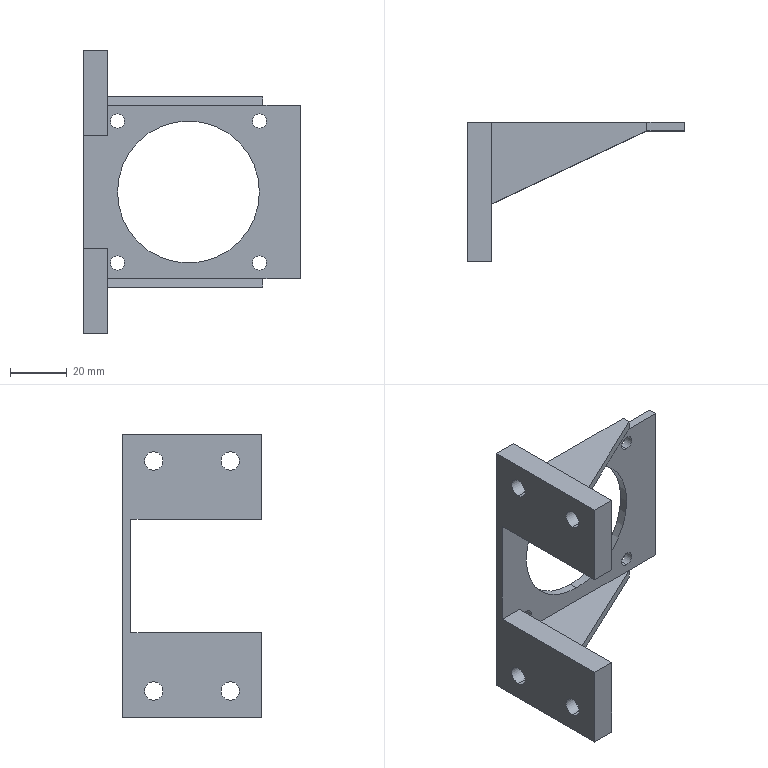Part | SolidWorks | features ICE 5, Extrusion 1, MirrorPattern 1 | 1 solid | 40 faces | box 76.5 x 49 x 100 mm | volume 36422 mm3 | plane 22 | cylinder 18 | commonest cylinder face diameters 5 x8 6.5 x8 50 x2
STEP:
#1=CARTESIAN_POINT('',(12.,24.5,-22.5));
#2=VERTEX_POINT('',#1);
#3=CARTESIAN_POINT('',(12.,24.5,-27.5));
#4=VERTEX_POINT('',#3);
#5=CARTESIAN_POINT('',(12.,24.5,-25.));
#6=DIRECTION('',(0.,-1.,0.));
#7=DIRECTION('',(0.,0.,-1.));
#8=AXIS2_PLACEMENT_3D('',#5,#6,#7);
#9=CIRCLE('',#8,2.5);
#10=EDGE_CURVE('',#2,#4,#9,.T.);
#11=ORIENTED_EDGE('',*,*,#10,.F.);
#12=CARTESIAN_POINT('',(12.,21.5,-22.5));
#13=VERTEX_POINT('',#12);
#14=CARTESIAN_POINT('',(12.,89.5,-22.5));
#15=DIRECTION('',(0.,-1.,0.));
#16=VECTOR('',#15,1000.);
#17=LINE('',#14,#16);
#18=EDGE_CURVE('',#2,#13,#17,.T.);
#19=ORIENTED_EDGE('',*,*,#18,.T.);
#20=CARTESIAN_POINT('',(12.,21.5,-27.5));
#21=VERTEX_POINT('',#20);
#22=CARTESIAN_POINT('',(12.,21.5,-25.));
#23=DIRECTION('',(0.,-1.,0.));
#24=DIRECTION('',(0.,0.,-1.));
#25=AXIS2_PLACEMENT_3D('',#22,#23,#24);
#26=CIRCLE('',#25,2.5);
#27=EDGE_CURVE('',#13,#21,#26,.T.);
#28=ORIENTED_EDGE('',*,*,#27,.T.);
#29=CARTESIAN_POINT('',(12.,89.5,-27.5));
#30=DIRECTION('',(0.,-1.,0.));
#31=VECTOR('',#30,1000.);
#32=LINE('',#29,#31);
#33=EDGE_CURVE('',#4,#21,#32,.T.);
#34=ORIENTED_EDGE('',*,*,#33,.F.);
#35=EDGE_LOOP('',(#11,#19,#28,#34));
#36=FACE_OUTER_BOUND('',#35,.T.);
#37=CARTESIAN_POINT('',(12.,89.5,-25.));
#38=DIRECTION('',(0.,-1.,0.));
#39=DIRECTION('',(0.,0.,-1.));
#40=AXIS2_PLACEMENT_3D('',#37,#38,#39);
#41=CYLINDRICAL_SURFACE('',#40,2.5);
#42=ADVANCED_FACE('',(#36),#41,.F.);
#43=CARTESIAN_POINT('',(62.,24.5,-22.5));
#44=VERTEX_POINT('',#43);
#45=CARTESIAN_POINT('',(62.,24.5,-27.5));
#46=VERTEX_POINT('',#45);
#47=CARTESIAN_POINT('',(62.,24.5,-25.));
#48=DIRECTION('',(0.,-1.,0.));
#49=DIRECTION('',(0.,0.,-1.));
#50=AXIS2_PLACEMENT_3D('',#47,#48,#49);
#51=CIRCLE('',#50,2.5);
#52=EDGE_CURVE('',#44,#46,#51,.T.);
#53=ORIENTED_EDGE('',*,*,#52,.F.);
#54=CARTESIAN_POINT('',(62.,21.5,-22.5));
#55=VERTEX_POINT('',#54);
#56=CARTESIAN_POINT('',(62.,89.5,-22.5));
#57=DIRECTION('',(0.,-1.,0.));
#58=VECTOR('',#57,1000.);
#59=LINE('',#56,#58);
#60=EDGE_CURVE('',#44,#55,#59,.T.);
#61=ORIENTED_EDGE('',*,*,#60,.T.);
#62=CARTESIAN_POINT('',(62.,21.5,-27.5));
#63=VERTEX_POINT('',#62);
#64=CARTESIAN_POINT('',(62.,21.5,-25.));
#65=DIRECTION('',(0.,-1.,0.));
#66=DIRECTION('',(0.,0.,-1.));
#67=AXIS2_PLACEMENT_3D('',#64,#65,#66);
#68=CIRCLE('',#67,2.5);
#69=EDGE_CURVE('',#55,#63,#68,.T.);
#70=ORIENTED_EDGE('',*,*,#69,.T.);
#71=CARTESIAN_POINT('',(62.,89.5,-27.5));
#72=DIRECTION('',(0.,-1.,0.));
#73=VECTOR('',#72,1000.);
#74=LINE('',#71,#73);
#75=EDGE_CURVE('',#46,#63,#74,.T.);
#76=ORIENTED_EDGE('',*,*,#75,.F.);
#77=EDGE_LOOP('',(#53,#61,#70,#76));
#78=FACE_OUTER_BOUND('',#77,.T.);
#79=CARTESIAN_POINT('',(62.,89.5,-25.));
#80=DIRECTION('',(0.,-1.,0.));
#81=DIRECTION('',(0.,0.,-1.));
#82=AXIS2_PLACEMENT_3D('',#79,#80,#81);
#83=CYLINDRICAL_SURFACE('',#82,2.5);
#84=ADVANCED_FACE('',(#78),#83,.F.);
#85=CARTESIAN_POINT('',(62.,24.5,27.5));
#86=VERTEX_POINT('',#85);
#87=CARTESIAN_POINT('',(62.,24.5,22.5));
#88=VERTEX_POINT('',#87);
#89=CARTESIAN_POINT('',(62.,24.5,25.));
#90=DIRECTION('',(0.,-1.,0.));
#91=DIRECTION('',(0.,0.,-1.));
#92=AXIS2_PLACEMENT_3D('',#89,#90,#91);
#93=CIRCLE('',#92,2.5);
#94=EDGE_CURVE('',#86,#88,#93,.T.);
#95=ORIENTED_EDGE('',*,*,#94,.F.);
#96=CARTESIAN_POINT('',(62.,21.5,27.5));
#97=VERTEX_POINT('',#96);
#98=CARTESIAN_POINT('',(62.,89.5,27.5));
#99=DIRECTION('',(0.,-1.,0.));
#100=VECTOR('',#99,1000.);
#101=LINE('',#98,#100);
#102=EDGE_CURVE('',#86,#97,#101,.T.);
#103=ORIENTED_EDGE('',*,*,#102,.T.);
#104=CARTESIAN_POINT('',(62.,21.5,22.5));
#105=VERTEX_POINT('',#104);
#106=CARTESIAN_POINT('',(62.,21.5,25.));
#107=DIRECTION('',(0.,-1.,0.));
#108=DIRECTION('',(0.,0.,-1.));
#109=AXIS2_PLACEMENT_3D('',#106,#107,#108);
#110=CIRCLE('',#109,2.5);
#111=EDGE_CURVE('',#97,#105,#110,.T.);
#112=ORIENTED_EDGE('',*,*,#111,.T.);
#113=CARTESIAN_POINT('',(62.,89.5,22.5));
#114=DIRECTION('',(0.,-1.,0.));
#115=VECTOR('',#114,1000.);
#116=LINE('',#113,#115);
#117=EDGE_CURVE('',#88,#105,#116,.T.);
#118=ORIENTED_EDGE('',*,*,#117,.F.);
#119=EDGE_LOOP('',(#95,#103,#112,#118));
#120=FACE_OUTER_BOUND('',#119,.T.);
#121=CARTESIAN_POINT('',(62.,89.5,25.));
#122=DIRECTION('',(0.,-1.,0.));
#123=DIRECTION('',(0.,0.,-1.));
#124=AXIS2_PLACEMENT_3D('',#121,#122,#123);
#125=CYLINDRICAL_SURFACE('',#124,2.5);
#126=ADVANCED_FACE('',(#120),#125,.F.);
#127=CARTESIAN_POINT('',(12.,24.5,27.5));
#128=VERTEX_POINT('',#127);
#129=CARTESIAN_POINT('',(12.,24.5,22.5));
#130=VERTEX_POINT('',#129);
#131=CARTESIAN_POINT('',(12.,24.5,25.));
#132=DIRECTION('',(0.,-1.,0.));
#133=DIRECTION('',(0.,0.,-1.));
#134=AXIS2_PLACEMENT_3D('',#131,#132,#133);
#135=CIRCLE('',#134,2.5);
#136=EDGE_CURVE('',#128,#130,#135,.T.);
#137=ORIENTED_EDGE('',*,*,#136,.F.);
#138=CARTESIAN_POINT('',(12.,21.5,27.5));
#139=VERTEX_POINT('',#138);
#140=CARTESIAN_POINT('',(12.,89.5,27.5));
#141=DIRECTION('',(0.,-1.,0.));
#142=VECTOR('',#141,1000.);
#143=LINE('',#140,#142);
#144=EDGE_CURVE('',#128,#139,#143,.T.);
#145=ORIENTED_EDGE('',*,*,#144,.T.);
#146=CARTESIAN_POINT('',(12.,21.5,22.5));
#147=VERTEX_POINT('',#146);
#148=CARTESIAN_POINT('',(12.,21.5,25.));
#149=DIRECTION('',(0.,-1.,0.));
#150=DIRECTION('',(0.,0.,-1.));
#151=AXIS2_PLACEMENT_3D('',#148,#149,#150);
#152=CIRCLE('',#151,2.5);
#153=EDGE_CURVE('',#139,#147,#152,.T.);
#154=ORIENTED_EDGE('',*,*,#153,.T.);
#155=CARTESIAN_POINT('',(12.,89.5,22.5));
#156=DIRECTION('',(0.,-1.,0.));
#157=VECTOR('',#156,1000.);
#158=LINE('',#155,#157);
#159=EDGE_CURVE('',#130,#147,#158,.T.);
#160=ORIENTED_EDGE('',*,*,#159,.F.);
#161=EDGE_LOOP('',(#137,#145,#154,#160));
#162=FACE_OUTER_BOUND('',#161,.T.);
#163=CARTESIAN_POINT('',(12.,89.5,25.));
#164=DIRECTION('',(0.,-1.,0.));
#165=DIRECTION('',(0.,0.,-1.));
#166=AXIS2_PLACEMENT_3D('',#163,#164,#165);
#167=CYLINDRICAL_SURFACE('',#166,2.5);
#168=ADVANCED_FACE('',(#162),#167,.F.);
#169=CARTESIAN_POINT('',(37.,24.5,25.));
#170=VERTEX_POINT('',#169);
#171=CARTESIAN_POINT('',(37.,24.5,-25.));
#172=VERTEX_POINT('',#171);
#173=CARTESIAN_POINT('',(37.,24.5,0.));
#174=DIRECTION('',(0.,-1.,0.));
#175=DIRECTION('',(0.,0.,-1.));
#176=AXIS2_PLACEMENT_3D('',#173,#174,#175);
#177=CIRCLE('',#176,25.);
#178=EDGE_CURVE('',#170,#172,#177,.T.);
#179=ORIENTED_EDGE('',*,*,#178,.F.);
#180=CARTESIAN_POINT('',(37.,21.5,25.));
#181=VERTEX_POINT('',#180);
#182=CARTESIAN_POINT('',(37.,89.5,25.));
#183=DIRECTION('',(0.,-1.,0.));
#184=VECTOR('',#183,1000.);
#185=LINE('',#182,#184);
#186=EDGE_CURVE('',#170,#181,#185,.T.);
#187=ORIENTED_EDGE('',*,*,#186,.T.);
#188=CARTESIAN_POINT('',(37.,21.5,-25.));
#189=VERTEX_POINT('',#188);
#190=CARTESIAN_POINT('',(37.,21.5,0.));
#191=DIRECTION('',(0.,-1.,0.));
#192=DIRECTION('',(0.,0.,-1.));
#193=AXIS2_PLACEMENT_3D('',#190,#191,#192);
#194=CIRCLE('',#193,25.);
#195=EDGE_CURVE('',#181,#189,#194,.T.);
#196=ORIENTED_EDGE('',*,*,#195,.T.);
#197=CARTESIAN_POINT('',(37.,89.5,-25.));
#198=DIRECTION('',(0.,-1.,0.));
#199=VECTOR('',#198,1000.);
#200=LINE('',#197,#199);
#201=EDGE_CURVE('',#172,#189,#200,.T.);
#202=ORIENTED_EDGE('',*,*,#201,.F.);
#203=EDGE_LOOP('',(#179,#187,#196,#202));
#204=FACE_OUTER_BOUND('',#203,.T.);
#205=CARTESIAN_POINT('',(37.,89.5,0.));
#206=DIRECTION('',(0.,-1.,0.));
#207=DIRECTION('',(0.,0.,-1.));
#208=AXIS2_PLACEMENT_3D('',#205,#206,#207);
#209=CYLINDRICAL_SURFACE('',#208,25.);
#210=ADVANCED_FACE('',(#204),#209,.F.);
#211=CARTESIAN_POINT('',(8.5,-13.5,43.75));
#212=VERTEX_POINT('',#211);
#213=CARTESIAN_POINT('',(8.5,-13.5,37.25));
#214=VERTEX_POINT('',#213);
#215=CARTESIAN_POINT('',(8.5,-13.5,40.5));
#216=DIRECTION('',(1.,0.,0.));
#217=DIRECTION('',(0.,0.,-1.));
#218=AXIS2_PLACEMENT_3D('',#215,#216,#217);
#219=CIRCLE('',#218,3.25);
#220=EDGE_CURVE('',#212,#214,#219,.T.);
#221=ORIENTED_EDGE('',*,*,#220,.T.);
#222=CARTESIAN_POINT('',(0.,-13.5,37.25));
#223=VERTEX_POINT('',#222);
#224=CARTESIAN_POINT('',(8.5,-13.5,37.25));
#225=DIRECTION('',(-1.,0.,0.));
#226=VECTOR('',#225,1000.);
#227=LINE('',#224,#226);
#228=EDGE_CURVE('',#214,#223,#227,.T.);
#229=ORIENTED_EDGE('',*,*,#228,.T.);
#230=CARTESIAN_POINT('',(0.,-13.5,43.75));
#231=VERTEX_POINT('',#230);
#232=CARTESIAN_POINT('',(0.,-13.5,40.5));
#233=DIRECTION('',(1.,0.,0.));
#234=DIRECTION('',(0.,0.,-1.));
#235=AXIS2_PLACEMENT_3D('',#232,#233,#234);
#236=CIRCLE('',#235,3.25);
#237=EDGE_CURVE('',#231,#223,#236,.T.);
#238=ORIENTED_EDGE('',*,*,#237,.F.);
#239=CARTESIAN_POINT('',(8.5,-13.5,43.75));
#240=DIRECTION('',(-1.,0.,0.));
#241=VECTOR('',#240,1000.);
#242=LINE('',#239,#241);
#243=EDGE_CURVE('',#212,#231,#242,.T.);
#244=ORIENTED_EDGE('',*,*,#243,.F.);
#245=EDGE_LOOP('',(#221,#229,#238,#244));
#246=FACE_OUTER_BOUND('',#245,.T.);
#247=CARTESIAN_POINT('',(8.5,-13.5,40.5));
#248=DIRECTION('',(-1.,0.,0.));
#249=DIRECTION('',(0.,0.,1.));
#250=AXIS2_PLACEMENT_3D('',#247,#248,#249);
#251=CYLINDRICAL_SURFACE('',#250,3.25);
#252=ADVANCED_FACE('',(#246),#251,.F.);
#253=CARTESIAN_POINT('',(8.5,-13.5,-37.25));
#254=VERTEX_POINT('',#253);
#255=CARTESIAN_POINT('',(8.5,-13.5,-43.75));
#256=VERTEX_POINT('',#255);
#257=CARTESIAN_POINT('',(8.5,-13.5,-40.5));
#258=DIRECTION('',(1.,0.,0.));
#259=DIRECTION('',(0.,0.,-1.));
#260=AXIS2_PLACEMENT_3D('',#257,#258,#259);
#261=CIRCLE('',#260,3.25);
#262=EDGE_CURVE('',#254,#256,#261,.T.);
#263=ORIENTED_EDGE('',*,*,#262,.T.);
#264=CARTESIAN_POINT('',(0.,-13.5,-43.75));
#265=VERTEX_POINT('',#264);
#266=CARTESIAN_POINT('',(8.5,-13.5,-43.75));
#267=DIRECTION('',(-1.,0.,0.));
#268=VECTOR('',#267,1000.);
#269=LINE('',#266,#268);
#270=EDGE_CURVE('',#256,#265,#269,.T.);
#271=ORIENTED_EDGE('',*,*,#270,.T.);
#272=CARTESIAN_POINT('',(0.,-13.5,-37.25));
#273=VERTEX_POINT('',#272);
#274=CARTESIAN_POINT('',(0.,-13.5,-40.5));
#275=DIRECTION('',(1.,0.,0.));
#276=DIRECTION('',(0.,0.,-1.));
#277=AXIS2_PLACEMENT_3D('',#274,#275,#276);
#278=CIRCLE('',#277,3.25);
#279=EDGE_CURVE('',#273,#265,#278,.T.);
#280=ORIENTED_EDGE('',*,*,#279,.F.);
#281=CARTESIAN_POINT('',(8.5,-13.5,-37.25));
#282=DIRECTION('',(-1.,0.,0.));
#283=VECTOR('',#282,1000.);
#284=LINE('',#281,#283);
#285=EDGE_CURVE('',#254,#273,#284,.T.);
#286=ORIENTED_EDGE('',*,*,#285,.F.);
#287=EDGE_LOOP('',(#263,#271,#280,#286));
#288=FACE_OUTER_BOUND('',#287,.T.);
#289=CARTESIAN_POINT('',(8.5,-13.5,-40.5));
#290=DIRECTION('',(-1.,0.,0.));
#291=DIRECTION('',(0.,0.,1.));
#292=AXIS2_PLACEMENT_3D('',#289,#290,#291);
#293=CYLINDRICAL_SURFACE('',#292,3.25);
#294=ADVANCED_FACE('',(#288),#293,.F.);
#295=CARTESIAN_POINT('',(8.5,13.5,-37.25));
#296=VERTEX_POINT('',#295);
#297=CARTESIAN_POINT('',(8.5,13.5,-43.75));
#298=VERTEX_POINT('',#297);
#299=CARTESIAN_POINT('',(8.5,13.5,-40.5));
#300=DIRECTION('',(1.,0.,0.));
#301=DIRECTION('',(0.,0.,-1.));
#302=AXIS2_PLACEMENT_3D('',#299,#300,#301);
#303=CIRCLE('',#302,3.25);
#304=EDGE_CURVE('',#296,#298,#303,.T.);
#305=ORIENTED_EDGE('',*,*,#304,.T.);
#306=CARTESIAN_POINT('',(0.,13.5,-43.75));
#307=VERTEX_POINT('',#306);
#308=CARTESIAN_POINT('',(8.5,13.5,-43.75));
#309=DIRECTION('',(-1.,0.,0.));
#310=VECTOR('',#309,1000.);
#311=LINE('',#308,#310);
#312=EDGE_CURVE('',#298,#307,#311,.T.);
#313=ORIENTED_EDGE('',*,*,#312,.T.);
#314=CARTESIAN_POINT('',(0.,13.5,-37.25));
#315=VERTEX_POINT('',#314);
#316=CARTESIAN_POINT('',(0.,13.5,-40.5));
#317=DIRECTION('',(1.,0.,0.));
#318=DIRECTION('',(0.,0.,-1.));
#319=AXIS2_PLACEMENT_3D('',#316,#317,#318);
#320=CIRCLE('',#319,3.25);
#321=EDGE_CURVE('',#315,#307,#320,.T.);
#322=ORIENTED_EDGE('',*,*,#321,.F.);
#323=CARTESIAN_POINT('',(8.5,13.5,-37.25));
#324=DIRECTION('',(-1.,0.,0.));
#325=VECTOR('',#324,1000.);
#326=LINE('',#323,#325);
#327=EDGE_CURVE('',#296,#315,#326,.T.);
#328=ORIENTED_EDGE('',*,*,#327,.F.);
#329=EDGE_LOOP('',(#305,#313,#322,#328));
#330=FACE_OUTER_BOUND('',#329,.T.);
#331=CARTESIAN_POINT('',(8.5,13.5,-40.5));
#332=DIRECTION('',(-1.,0.,0.));
#333=DIRECTION('',(0.,0.,1.));
#334=AXIS2_PLACEMENT_3D('',#331,#332,#333);
#335=CYLINDRICAL_SURFACE('',#334,3.25);
#336=ADVANCED_FACE('',(#330),#335,.F.);
#337=CARTESIAN_POINT('',(8.5,13.5,43.75));
#338=VERTEX_POINT('',#337);
#339=CARTESIAN_POINT('',(8.5,13.5,37.25));
#340=VERTEX_POINT('',#339);
#341=CARTESIAN_POINT('',(8.5,13.5,40.5));
#342=DIRECTION('',(1.,0.,0.));
#343=DIRECTION('',(0.,0.,-1.));
#344=AXIS2_PLACEMENT_3D('',#341,#342,#343);
#345=CIRCLE('',#344,3.25);
#346=EDGE_CURVE('',#338,#340,#345,.T.);
#347=ORIENTED_EDGE('',*,*,#346,.T.);
#348=CARTESIAN_POINT('',(0.,13.5,37.25));
#349=VERTEX_POINT('',#348);
#350=CARTESIAN_POINT('',(8.5,13.5,37.25));
#351=DIRECTION('',(-1.,0.,0.));
#352=VECTOR('',#351,1000.);
#353=LINE('',#350,#352);
#354=EDGE_CURVE('',#340,#349,#353,.T.);
#355=ORIENTED_EDGE('',*,*,#354,.T.);
#356=CARTESIAN_POINT('',(0.,13.5,43.75));
#357=VERTEX_POINT('',#356);
#358=CARTESIAN_POINT('',(0.,13.5,40.5));
#359=DIRECTION('',(1.,0.,0.));
#360=DIRECTION('',(0.,0.,-1.));
#361=AXIS2_PLACEMENT_3D('',#358,#359,#360);
#362=CIRCLE('',#361,3.25);
#363=EDGE_CURVE('',#357,#349,#362,.T.);
#364=ORIENTED_EDGE('',*,*,#363,.F.);
#365=CARTESIAN_POINT('',(8.5,13.5,43.75));
#366=DIRECTION('',(-1.,0.,0.));
#367=VECTOR('',#366,1000.);
#368=LINE('',#365,#367);
#369=EDGE_CURVE('',#338,#357,#368,.T.);
#370=ORIENTED_EDGE('',*,*,#369,.F.);
#371=EDGE_LOOP('',(#347,#355,#364,#370));
#372=FACE_OUTER_BOUND('',#371,.T.);
#373=CARTESIAN_POINT('',(8.5,13.5,40.5));
#374=DIRECTION('',(-1.,0.,0.));
#375=DIRECTION('',(0.,0.,1.));
#376=AXIS2_PLACEMENT_3D('',#373,#374,#375);
#377=CYLINDRICAL_SURFACE('',#376,3.25);
#378=ADVANCED_FACE('',(#372),#377,.F.);
#379=CARTESIAN_POINT('',(63.24,24.5,-30.5));
#380=VERTEX_POINT('',#379);
#381=CARTESIAN_POINT('',(63.24,21.5,-30.5));
#382=VERTEX_POINT('',#381);
#383=CARTESIAN_POINT('',(63.24,24.5,-30.5));
#384=DIRECTION('',(0.,-1.,0.));
#385=VECTOR('',#384,1000.);
#386=LINE('',#383,#385);
#387=EDGE_CURVE('',#380,#382,#386,.T.);
#388=ORIENTED_EDGE('',*,*,#387,.F.);
#389=CARTESIAN_POINT('',(76.5,24.5,-30.5));
#390=VERTEX_POINT('',#389);
#391=CARTESIAN_POINT('',(76.5,24.5,-30.5));
#392=DIRECTION('',(-1.,0.,0.));
#393=VECTOR('',#392,1000.);
#394=LINE('',#391,#393);
#395=EDGE_CURVE('',#390,#380,#394,.T.);
#396=ORIENTED_EDGE('',*,*,#395,.F.);
#397=CARTESIAN_POINT('',(76.5,21.5,-30.5));
#398=VERTEX_POINT('',#397);
#399=CARTESIAN_POINT('',(76.5,21.5,-30.5));
#400=DIRECTION('',(0.,1.,0.));
#401=VECTOR('',#400,1000.);
#402=LINE('',#399,#401);
#403=EDGE_CURVE('',#398,#390,#402,.T.);
#404=ORIENTED_EDGE('',*,*,#403,.F.);
#405=CARTESIAN_POINT('',(76.5,21.5,-30.5));
#406=DIRECTION('',(-1.,0.,0.));
#407=VECTOR('',#406,1000.);
#408=LINE('',#405,#407);
#409=EDGE_CURVE('',#398,#382,#408,.T.);
#410=ORIENTED_EDGE('',*,*,#409,.T.);
#411=EDGE_LOOP('',(#388,#396,#404,#410));
#412=FACE_OUTER_BOUND('',#411,.T.);
#413=CARTESIAN_POINT('',(76.5,21.5,-30.5));
#414=DIRECTION('',(0.,0.,1.));
#415=DIRECTION('',(1.,0.,0.));
#416=AXIS2_PLACEMENT_3D('',#413,#414,#415);
#417=PLANE('',#416);
#418=ADVANCED_FACE('',(#412),#417,.F.);
#419=CARTESIAN_POINT('',(8.5,-4.299,33.5));
#420=VERTEX_POINT('',#419);
#421=CARTESIAN_POINT('',(8.5,24.5,33.5));
#422=VERTEX_POINT('',#421);
#423=CARTESIAN_POINT('',(8.5,-4.299,33.5));
#424=DIRECTION('',(0.,1.,0.));
#425=VECTOR('',#424,1000.);
#426=LINE('',#423,#425);
#427=EDGE_CURVE('',#420,#422,#426,.T.);
#428=ORIENTED_EDGE('',*,*,#427,.T.);
#429=CARTESIAN_POINT('',(8.5,24.5,50.));
#430=VERTEX_POINT('',#429);
#431=CARTESIAN_POINT('',(8.5,24.5,-50.));
#432=DIRECTION('',(0.,0.,1.));
#433=VECTOR('',#432,1000.);
#434=LINE('',#431,#433);
#435=EDGE_CURVE('',#422,#430,#434,.T.);
#436=ORIENTED_EDGE('',*,*,#435,.T.);
#437=CARTESIAN_POINT('',(8.5,-24.5,50.));
#438=VERTEX_POINT('',#437);
#439=CARTESIAN_POINT('',(8.5,-24.5,50.));
#440=DIRECTION('',(0.,-1.,0.));
#441=VECTOR('',#440,1000.);
#442=LINE('',#439,#441);
#443=EDGE_CURVE('',#430,#438,#442,.T.);
#444=ORIENTED_EDGE('',*,*,#443,.T.);
#445=CARTESIAN_POINT('',(8.5,-24.5,20.));
#446=VERTEX_POINT('',#445);
#447=CARTESIAN_POINT('',(8.5,-24.5,-50.));
#448=DIRECTION('',(0.,0.,-1.));
#449=VECTOR('',#448,1000.);
#450=LINE('',#447,#449);
#451=EDGE_CURVE('',#438,#446,#450,.T.);
#452=ORIENTED_EDGE('',*,*,#451,.T.);
#453=CARTESIAN_POINT('',(8.5,21.5,20.));
#454=VERTEX_POINT('',#453);
#455=CARTESIAN_POINT('',(8.5,-24.5,20.));
#456=DIRECTION('',(0.,-1.,0.));
#457=VECTOR('',#456,1000.);
#458=LINE('',#455,#457);
#459=EDGE_CURVE('',#454,#446,#458,.T.);
#460=ORIENTED_EDGE('',*,*,#459,.F.);
#461=CARTESIAN_POINT('',(8.5,21.5,30.5));
#462=VERTEX_POINT('',#461);
#463=CARTESIAN_POINT('',(8.5,21.5,-30.5));
#464=DIRECTION('',(0.,0.,-1.));
#465=VECTOR('',#464,1000.);
#466=LINE('',#463,#465);
#467=EDGE_CURVE('',#462,#454,#466,.T.);
#468=ORIENTED_EDGE('',*,*,#467,.F.);
#469=CARTESIAN_POINT('',(8.5,-4.299,30.5));
#470=VERTEX_POINT('',#469);
#471=CARTESIAN_POINT('',(8.5,-4.299,30.5));
#472=DIRECTION('',(0.,1.,0.));
#473=VECTOR('',#472,1000.);
#474=LINE('',#471,#473);
#475=EDGE_CURVE('',#470,#462,#474,.T.);
#476=ORIENTED_EDGE('',*,*,#475,.F.);
#477=CARTESIAN_POINT('',(8.5,-4.299,33.5));
#478=DIRECTION('',(0.,0.,-1.));
#479=VECTOR('',#478,1000.);
#480=LINE('',#477,#479);
#481=EDGE_CURVE('',#420,#470,#480,.T.);
#482=ORIENTED_EDGE('',*,*,#481,.F.);
#483=EDGE_LOOP('',(#428,#436,#444,#452,#460,#468,#476,#482));
#484=FACE_OUTER_BOUND('',#483,.T.);
#485=ORIENTED_EDGE('',*,*,#220,.F.);
#486=CARTESIAN_POINT('',(8.5,-13.5,40.5));
#487=DIRECTION('',(1.,0.,0.));
#488=DIRECTION('',(0.,0.,-1.));
#489=AXIS2_PLACEMENT_3D('',#486,#487,#488);
#490=CIRCLE('',#489,3.25);
#491=EDGE_CURVE('',#214,#212,#490,.T.);
#492=ORIENTED_EDGE('',*,*,#491,.F.);
#493=EDGE_LOOP('',(#485,#492));
#494=FACE_BOUND('',#493,.T.);
#495=ORIENTED_EDGE('',*,*,#346,.F.);
#496=CARTESIAN_POINT('',(8.5,13.5,40.5));
#497=DIRECTION('',(1.,0.,0.));
#498=DIRECTION('',(0.,0.,-1.));
#499=AXIS2_PLACEMENT_3D('',#496,#497,#498);
#500=CIRCLE('',#499,3.25);
#501=EDGE_CURVE('',#340,#338,#500,.T.);
#502=ORIENTED_EDGE('',*,*,#501,.F.);
#503=EDGE_LOOP('',(#495,#502));
#504=FACE_BOUND('',#503,.T.);
#505=CARTESIAN_POINT('',(8.5,0.,0.));
#506=DIRECTION('',(1.,0.,0.));
#507=DIRECTION('',(0.,0.,-1.));
#508=AXIS2_PLACEMENT_3D('',#505,#506,#507);
#509=PLANE('',#508);
#510=ADVANCED_FACE('',(#484,#494,#504),#509,.T.);
#511=CARTESIAN_POINT('',(0.,-24.5,50.));
#512=VERTEX_POINT('',#511);
#513=CARTESIAN_POINT('',(0.,-24.5,20.));
#514=VERTEX_POINT('',#513);
#515=CARTESIAN_POINT('',(0.,-24.5,-50.));
#516=DIRECTION('',(0.,0.,-1.));
#517=VECTOR('',#516,1000.);
#518=LINE('',#515,#517);
#519=EDGE_CURVE('',#512,#514,#518,.T.);
#520=ORIENTED_EDGE('',*,*,#519,.T.);
#521=CARTESIAN_POINT('',(8.5,-24.5,20.));
#522=DIRECTION('',(1.,0.,0.));
#523=VECTOR('',#522,1000.);
#524=LINE('',#521,#523);
#525=EDGE_CURVE('',#514,#446,#524,.T.);
#526=ORIENTED_EDGE('',*,*,#525,.T.);
#527=ORIENTED_EDGE('',*,*,#451,.F.);
#528=CARTESIAN_POINT('',(8.5,-24.5,50.));
#529=DIRECTION('',(-1.,0.,0.));
#530=VECTOR('',#529,1000.);
#531=LINE('',#528,#530);
#532=EDGE_CURVE('',#438,#512,#531,.T.);
#533=ORIENTED_EDGE('',*,*,#532,.T.);
#534=EDGE_LOOP('',(#520,#526,#527,#533));
#535=FACE_OUTER_BOUND('',#534,.T.);
#536=CARTESIAN_POINT('',(8.5,-24.5,-50.));
#537=DIRECTION('',(0.,1.,0.));
#538=DIRECTION('',(0.,0.,1.));
#539=AXIS2_PLACEMENT_3D('',#536,#537,#538);
#540=PLANE('',#539);
#541=ADVANCED_FACE('',(#535),#540,.F.);
#542=CARTESIAN_POINT('',(8.5,-4.299,-33.5));
#543=VERTEX_POINT('',#542);
#544=CARTESIAN_POINT('',(8.5,24.5,-33.5));
#545=VERTEX_POINT('',#544);
#546=CARTESIAN_POINT('',(8.5,-4.299,-33.5));
#547=DIRECTION('',(0.,1.,0.));
#548=VECTOR('',#547,1000.);
#549=LINE('',#546,#548);
#550=EDGE_CURVE('',#543,#545,#549,.T.);
#551=ORIENTED_EDGE('',*,*,#550,.F.);
#552=CARTESIAN_POINT('',(8.5,-4.299,-30.5));
#553=VERTEX_POINT('',#552);
#554=CARTESIAN_POINT('',(8.5,-4.299,-33.5));
#555=DIRECTION('',(0.,0.,1.));
#556=VECTOR('',#555,1000.);
#557=LINE('',#554,#556);
#558=EDGE_CURVE('',#543,#553,#557,.T.);
#559=ORIENTED_EDGE('',*,*,#558,.T.);
#560=CARTESIAN_POINT('',(8.5,21.5,-30.5));
#561=VERTEX_POINT('',#560);
#562=CARTESIAN_POINT('',(8.5,-4.299,-30.5));
#563=DIRECTION('',(0.,1.,0.));
#564=VECTOR('',#563,1000.);
#565=LINE('',#562,#564);
#566=EDGE_CURVE('',#553,#561,#565,.T.);
#567=ORIENTED_EDGE('',*,*,#566,.T.);
#568=CARTESIAN_POINT('',(8.5,21.5,-20.));
#569=VERTEX_POINT('',#568);
#570=CARTESIAN_POINT('',(8.5,21.5,-30.5));
#571=DIRECTION('',(0.,0.,-1.));
#572=VECTOR('',#571,1000.);
#573=LINE('',#570,#572);
#574=EDGE_CURVE('',#569,#561,#573,.T.);
#575=ORIENTED_EDGE('',*,*,#574,.F.);
#576=CARTESIAN_POINT('',(8.5,-24.5,-20.));
#577=VERTEX_POINT('',#576);
#578=CARTESIAN_POINT('',(8.5,-24.5,-20.));
#579=DIRECTION('',(0.,1.,0.));
#580=VECTOR('',#579,1000.);
#581=LINE('',#578,#580);
#582=EDGE_CURVE('',#577,#569,#581,.T.);
#583=ORIENTED_EDGE('',*,*,#582,.F.);
#584=CARTESIAN_POINT('',(8.5,-24.5,-50.));
#585=VERTEX_POINT('',#584);
#586=CARTESIAN_POINT('',(8.5,-24.5,-50.));
#587=DIRECTION('',(0.,0.,-1.));
#588=VECTOR('',#587,1000.);
#589=LINE('',#586,#588);
#590=EDGE_CURVE('',#577,#585,#589,.T.);
#591=ORIENTED_EDGE('',*,*,#590,.T.);
#592=CARTESIAN_POINT('',(8.5,24.5,-50.));
#593=VERTEX_POINT('',#592);
#594=CARTESIAN_POINT('',(8.5,-24.5,-50.));
#595=DIRECTION('',(0.,1.,0.));
#596=VECTOR('',#595,1000.);
#597=LINE('',#594,#596);
#598=EDGE_CURVE('',#585,#593,#597,.T.);
#599=ORIENTED_EDGE('',*,*,#598,.T.);
#600=CARTESIAN_POINT('',(8.5,24.5,-50.));
#601=DIRECTION('',(0.,0.,1.));
#602=VECTOR('',#601,1000.);
#603=LINE('',#600,#602);
#604=EDGE_CURVE('',#593,#545,#603,.T.);
#605=ORIENTED_EDGE('',*,*,#604,.T.);
#606=EDGE_LOOP('',(#551,#559,#567,#575,#583,#591,#599,#605));
#607=FACE_OUTER_BOUND('',#606,.T.);
#608=ORIENTED_EDGE('',*,*,#262,.F.);
#609=CARTESIAN_POINT('',(8.5,-13.5,-40.5));
#610=DIRECTION('',(1.,0.,0.));
#611=DIRECTION('',(0.,0.,-1.));
#612=AXIS2_PLACEMENT_3D('',#609,#610,#611);
#613=CIRCLE('',#612,3.25);
#614=EDGE_CURVE('',#256,#254,#613,.T.);
#615=ORIENTED_EDGE('',*,*,#614,.F.);
#616=EDGE_LOOP('',(#608,#615));
#617=FACE_BOUND('',#616,.T.);
#618=ORIENTED_EDGE('',*,*,#304,.F.);
#619=CARTESIAN_POINT('',(8.5,13.5,-40.5));
#620=DIRECTION('',(1.,0.,0.));
#621=DIRECTION('',(0.,0.,-1.));
#622=AXIS2_PLACEMENT_3D('',#619,#620,#621);
#623=CIRCLE('',#622,3.25);
#624=EDGE_CURVE('',#298,#296,#623,.T.);
#625=ORIENTED_EDGE('',*,*,#624,.F.);
#626=EDGE_LOOP('',(#618,#625));
#627=FACE_BOUND('',#626,.T.);
#628=CARTESIAN_POINT('',(8.5,0.,0.));
#629=DIRECTION('',(1.,0.,0.));
#630=DIRECTION('',(0.,0.,-1.));
#631=AXIS2_PLACEMENT_3D('',#628,#629,#630);
#632=PLANE('',#631);
#633=ADVANCED_FACE('',(#607,#617,#627),#632,.T.);
#634=CARTESIAN_POINT('',(0.,21.5,-20.));
#635=VERTEX_POINT('',#634);
#636=CARTESIAN_POINT('',(0.,21.5,20.));
#637=VERTEX_POINT('',#636);
#638=CARTESIAN_POINT('',(0.,21.5,0.));
#639=DIRECTION('',(0.,0.,1.));
#640=VECTOR('',#639,1000.);
#641=LINE('',#638,#640);
#642=EDGE_CURVE('',#635,#637,#641,.T.);
#643=ORIENTED_EDGE('',*,*,#642,.T.);
#644=CARTESIAN_POINT('',(0.,0.,20.));
#645=DIRECTION('',(0.,-1.,0.));
#646=VECTOR('',#645,1000.);
#647=LINE('',#644,#646);
#648=EDGE_CURVE('',#637,#514,#647,.T.);
#649=ORIENTED_EDGE('',*,*,#648,.T.);
#650=ORIENTED_EDGE('',*,*,#519,.F.);
#651=CARTESIAN_POINT('',(0.,24.5,50.));
#652=VERTEX_POINT('',#651);
#653=CARTESIAN_POINT('',(0.,-24.5,50.));
#654=DIRECTION('',(0.,-1.,0.));
#655=VECTOR('',#654,1000.);
#656=LINE('',#653,#655);
#657=EDGE_CURVE('',#652,#512,#656,.T.);
#658=ORIENTED_EDGE('',*,*,#657,.F.);
#659=CARTESIAN_POINT('',(0.,24.5,-50.));
#660=VERTEX_POINT('',#659);
#661=CARTESIAN_POINT('',(0.,24.5,-50.));
#662=DIRECTION('',(0.,0.,1.));
#663=VECTOR('',#662,1000.);
#664=LINE('',#661,#663);
#665=EDGE_CURVE('',#660,#652,#664,.T.);
#666=ORIENTED_EDGE('',*,*,#665,.F.);
#667=CARTESIAN_POINT('',(0.,-24.5,-50.));
#668=VERTEX_POINT('',#667);
#669=CARTESIAN_POINT('',(0.,-24.5,-50.));
#670=DIRECTION('',(0.,1.,0.));
#671=VECTOR('',#670,1000.);
#672=LINE('',#669,#671);
#673=EDGE_CURVE('',#668,#660,#672,.T.);
#674=ORIENTED_EDGE('',*,*,#673,.F.);
#675=CARTESIAN_POINT('',(0.,-24.5,-20.));
#676=VERTEX_POINT('',#675);
#677=CARTESIAN_POINT('',(0.,-24.5,-50.));
#678=DIRECTION('',(0.,0.,-1.));
#679=VECTOR('',#678,1000.);
#680=LINE('',#677,#679);
#681=EDGE_CURVE('',#676,#668,#680,.T.);
#682=ORIENTED_EDGE('',*,*,#681,.F.);
#683=CARTESIAN_POINT('',(0.,0.,-20.));
#684=DIRECTION('',(0.,1.,0.));
#685=VECTOR('',#684,1000.);
#686=LINE('',#683,#685);
#687=EDGE_CURVE('',#676,#635,#686,.T.);
#688=ORIENTED_EDGE('',*,*,#687,.T.);
#689=EDGE_LOOP('',(#643,#649,#650,#658,#666,#674,#682,#688));
#690=FACE_OUTER_BOUND('',#689,.T.);
#691=ORIENTED_EDGE('',*,*,#363,.T.);
#692=CARTESIAN_POINT('',(0.,13.5,40.5));
#693=DIRECTION('',(1.,0.,0.));
#694=DIRECTION('',(0.,0.,-1.));
#695=AXIS2_PLACEMENT_3D('',#692,#693,#694);
#696=CIRCLE('',#695,3.25);
#697=EDGE_CURVE('',#349,#357,#696,.T.);
#698=ORIENTED_EDGE('',*,*,#697,.T.);
#699=EDGE_LOOP('',(#691,#698));
#700=FACE_BOUND('',#699,.T.);
#701=ORIENTED_EDGE('',*,*,#321,.T.);
#702=CARTESIAN_POINT('',(0.,13.5,-40.5));
#703=DIRECTION('',(1.,0.,0.));
#704=DIRECTION('',(0.,0.,-1.));
#705=AXIS2_PLACEMENT_3D('',#702,#703,#704);
#706=CIRCLE('',#705,3.25);
#707=EDGE_CURVE('',#307,#315,#706,.T.);
#708=ORIENTED_EDGE('',*,*,#707,.T.);
#709=EDGE_LOOP('',(#701,#708));
#710=FACE_BOUND('',#709,.T.);
#711=ORIENTED_EDGE('',*,*,#279,.T.);
#712=CARTESIAN_POINT('',(0.,-13.5,-40.5));
#713=DIRECTION('',(1.,0.,0.));
#714=DIRECTION('',(0.,0.,-1.));
#715=AXIS2_PLACEMENT_3D('',#712,#713,#714);
#716=CIRCLE('',#715,3.25);
#717=EDGE_CURVE('',#265,#273,#716,.T.);
#718=ORIENTED_EDGE('',*,*,#717,.T.);
#719=EDGE_LOOP('',(#711,#718));
#720=FACE_BOUND('',#719,.T.);
#721=ORIENTED_EDGE('',*,*,#237,.T.);
#722=CARTESIAN_POINT('',(0.,-13.5,40.5));
#723=DIRECTION('',(1.,0.,0.));
#724=DIRECTION('',(0.,0.,-1.));
#725=AXIS2_PLACEMENT_3D('',#722,#723,#724);
#726=CIRCLE('',#725,3.25);
#727=EDGE_CURVE('',#223,#231,#726,.T.);
#728=ORIENTED_EDGE('',*,*,#727,.T.);
#729=EDGE_LOOP('',(#721,#728));
#730=FACE_BOUND('',#729,.T.);
#731=CARTESIAN_POINT('',(0.,0.,0.));
#732=DIRECTION('',(1.,0.,0.));
#733=DIRECTION('',(0.,0.,-1.));
#734=AXIS2_PLACEMENT_3D('',#731,#732,#733);
#735=PLANE('',#734);
#736=ADVANCED_FACE('',(#690,#700,#710,#720,#730),#735,.F.);
#737=ORIENTED_EDGE('',*,*,#657,.T.);
#738=ORIENTED_EDGE('',*,*,#532,.F.);
#739=ORIENTED_EDGE('',*,*,#443,.F.);
#740=CARTESIAN_POINT('',(8.5,24.5,50.));
#741=DIRECTION('',(-1.,0.,0.));
#742=VECTOR('',#741,1000.);
#743=LINE('',#740,#742);
#744=EDGE_CURVE('',#430,#652,#743,.T.);
#745=ORIENTED_EDGE('',*,*,#744,.T.);
#746=EDGE_LOOP('',(#737,#738,#739,#745));
#747=FACE_OUTER_BOUND('',#746,.T.);
#748=CARTESIAN_POINT('',(8.5,-24.5,50.));
#749=DIRECTION('',(0.,0.,-1.));
#750=DIRECTION('',(-1.,0.,0.));
#751=AXIS2_PLACEMENT_3D('',#748,#749,#750);
#752=PLANE('',#751);
#753=ADVANCED_FACE('',(#747),#752,.F.);
#754=ORIENTED_EDGE('',*,*,#590,.F.);
#755=CARTESIAN_POINT('',(8.5,-24.5,-20.));
#756=DIRECTION('',(-1.,0.,0.));
#757=VECTOR('',#756,1000.);
#758=LINE('',#755,#757);
#759=EDGE_CURVE('',#577,#676,#758,.T.);
#760=ORIENTED_EDGE('',*,*,#759,.T.);
#761=ORIENTED_EDGE('',*,*,#681,.T.);
#762=CARTESIAN_POINT('',(8.5,-24.5,-50.));
#763=DIRECTION('',(-1.,0.,0.));
#764=VECTOR('',#763,1000.);
#765=LINE('',#762,#764);
#766=EDGE_CURVE('',#585,#668,#765,.T.);
#767=ORIENTED_EDGE('',*,*,#766,.F.);
#768=EDGE_LOOP('',(#754,#760,#761,#767));
#769=FACE_OUTER_BOUND('',#768,.T.);
#770=CARTESIAN_POINT('',(8.5,-24.5,-50.));
#771=DIRECTION('',(0.,1.,0.));
#772=DIRECTION('',(0.,0.,1.));
#773=AXIS2_PLACEMENT_3D('',#770,#771,#772);
#774=PLANE('',#773);
#775=ADVANCED_FACE('',(#769),#774,.F.);
#776=ORIENTED_EDGE('',*,*,#673,.T.);
#777=CARTESIAN_POINT('',(8.5,24.5,-50.));
#778=DIRECTION('',(-1.,0.,0.));
#779=VECTOR('',#778,1000.);
#780=LINE('',#777,#779);
#781=EDGE_CURVE('',#593,#660,#780,.T.);
#782=ORIENTED_EDGE('',*,*,#781,.F.);
#783=ORIENTED_EDGE('',*,*,#598,.F.);
#784=ORIENTED_EDGE('',*,*,#766,.T.);
#785=EDGE_LOOP('',(#776,#782,#783,#784));
#786=FACE_OUTER_BOUND('',#785,.T.);
#787=CARTESIAN_POINT('',(8.5,-24.5,-50.));
#788=DIRECTION('',(0.,0.,1.));
#789=DIRECTION('',(1.,0.,0.));
#790=AXIS2_PLACEMENT_3D('',#787,#788,#789);
#791=PLANE('',#790);
#792=ADVANCED_FACE('',(#786),#791,.F.);
#793=ORIENTED_EDGE('',*,*,#435,.F.);
#794=CARTESIAN_POINT('',(63.24,24.5,33.5));
#795=VERTEX_POINT('',#794);
#796=CARTESIAN_POINT('',(8.5,24.5,33.5));
#797=DIRECTION('',(1.,0.,0.));
#798=VECTOR('',#797,1000.);
#799=LINE('',#796,#798);
#800=EDGE_CURVE('',#422,#795,#799,.T.);
#801=ORIENTED_EDGE('',*,*,#800,.T.);
#802=CARTESIAN_POINT('',(63.24,24.5,30.5));
#803=VERTEX_POINT('',#802);
#804=CARTESIAN_POINT('',(63.24,24.5,33.5));
#805=DIRECTION('',(0.,0.,-1.));
#806=VECTOR('',#805,1000.);
#807=LINE('',#804,#806);
#808=EDGE_CURVE('',#795,#803,#807,.T.);
#809=ORIENTED_EDGE('',*,*,#808,.T.);
#810=CARTESIAN_POINT('',(76.5,24.5,30.5));
#811=VERTEX_POINT('',#810);
#812=CARTESIAN_POINT('',(76.5,24.5,30.5));
#813=DIRECTION('',(-1.,0.,0.));
#814=VECTOR('',#813,1000.);
#815=LINE('',#812,#814);
#816=EDGE_CURVE('',#811,#803,#815,.T.);
#817=ORIENTED_EDGE('',*,*,#816,.F.);
#818=CARTESIAN_POINT('',(76.5,24.5,-30.5));
#819=DIRECTION('',(0.,0.,1.));
#820=VECTOR('',#819,1000.);
#821=LINE('',#818,#820);
#822=EDGE_CURVE('',#390,#811,#821,.T.);
#823=ORIENTED_EDGE('',*,*,#822,.F.);
#824=ORIENTED_EDGE('',*,*,#395,.T.);
#825=CARTESIAN_POINT('',(63.24,24.5,-33.5));
#826=VERTEX_POINT('',#825);
#827=CARTESIAN_POINT('',(63.24,24.5,-33.5));
#828=DIRECTION('',(0.,0.,1.));
#829=VECTOR('',#828,1000.);
#830=LINE('',#827,#829);
#831=EDGE_CURVE('',#826,#380,#830,.T.);
#832=ORIENTED_EDGE('',*,*,#831,.F.);
#833=CARTESIAN_POINT('',(8.5,24.5,-33.5));
#834=DIRECTION('',(1.,0.,0.));
#835=VECTOR('',#834,1000.);
#836=LINE('',#833,#835);
#837=EDGE_CURVE('',#545,#826,#836,.T.);
#838=ORIENTED_EDGE('',*,*,#837,.F.);
#839=ORIENTED_EDGE('',*,*,#604,.F.);
#840=ORIENTED_EDGE('',*,*,#781,.T.);
#841=ORIENTED_EDGE('',*,*,#665,.T.);
#842=ORIENTED_EDGE('',*,*,#744,.F.);
#843=EDGE_LOOP('',(#793,#801,#809,#817,#823,#824,#832,#838,#839,#840,#841,#842));
#844=FACE_OUTER_BOUND('',#843,.T.);
#845=CARTESIAN_POINT('',(12.,24.5,-25.));
#846=DIRECTION('',(0.,-1.,0.));
#847=DIRECTION('',(0.,0.,-1.));
#848=AXIS2_PLACEMENT_3D('',#845,#846,#847);
#849=CIRCLE('',#848,2.5);
#850=EDGE_CURVE('',#4,#2,#849,.T.);
#851=ORIENTED_EDGE('',*,*,#850,.T.);
#852=ORIENTED_EDGE('',*,*,#10,.T.);
#853=EDGE_LOOP('',(#851,#852));
#854=FACE_BOUND('',#853,.T.);
#855=CARTESIAN_POINT('',(62.,24.5,-25.));
#856=DIRECTION('',(0.,-1.,0.));
#857=DIRECTION('',(0.,0.,-1.));
#858=AXIS2_PLACEMENT_3D('',#855,#856,#857);
#859=CIRCLE('',#858,2.5);
#860=EDGE_CURVE('',#46,#44,#859,.T.);
#861=ORIENTED_EDGE('',*,*,#860,.T.);
#862=ORIENTED_EDGE('',*,*,#52,.T.);
#863=EDGE_LOOP('',(#861,#862));
#864=FACE_BOUND('',#863,.T.);
#865=CARTESIAN_POINT('',(62.,24.5,25.));
#866=DIRECTION('',(0.,-1.,0.));
#867=DIRECTION('',(0.,0.,-1.));
#868=AXIS2_PLACEMENT_3D('',#865,#866,#867);
#869=CIRCLE('',#868,2.5);
#870=EDGE_CURVE('',#88,#86,#869,.T.);
#871=ORIENTED_EDGE('',*,*,#870,.T.);
#872=ORIENTED_EDGE('',*,*,#94,.T.);
#873=EDGE_LOOP('',(#871,#872));
#874=FACE_BOUND('',#873,.T.);
#875=CARTESIAN_POINT('',(12.,24.5,25.));
#876=DIRECTION('',(0.,-1.,0.));
#877=DIRECTION('',(0.,0.,-1.));
#878=AXIS2_PLACEMENT_3D('',#875,#876,#877);
#879=CIRCLE('',#878,2.5);
#880=EDGE_CURVE('',#130,#128,#879,.T.);
#881=ORIENTED_EDGE('',*,*,#880,.T.);
#882=ORIENTED_EDGE('',*,*,#136,.T.);
#883=EDGE_LOOP('',(#881,#882));
#884=FACE_BOUND('',#883,.T.);
#885=CARTESIAN_POINT('',(37.,24.5,0.));
#886=DIRECTION('',(0.,-1.,0.));
#887=DIRECTION('',(0.,0.,-1.));
#888=AXIS2_PLACEMENT_3D('',#885,#886,#887);
#889=CIRCLE('',#888,25.);
#890=EDGE_CURVE('',#172,#170,#889,.T.);
#891=ORIENTED_EDGE('',*,*,#890,.T.);
#892=ORIENTED_EDGE('',*,*,#178,.T.);
#893=EDGE_LOOP('',(#891,#892));
#894=FACE_BOUND('',#893,.T.);
#895=CARTESIAN_POINT('',(8.5,24.5,-50.));
#896=DIRECTION('',(0.,-1.,0.));
#897=DIRECTION('',(0.,0.,-1.));
#898=AXIS2_PLACEMENT_3D('',#895,#896,#897);
#899=PLANE('',#898);
#900=ADVANCED_FACE('',(#844,#854,#864,#874,#884,#894),#899,.F.);
#901=ORIENTED_EDGE('',*,*,#354,.F.);
#902=ORIENTED_EDGE('',*,*,#501,.T.);
#903=ORIENTED_EDGE('',*,*,#369,.T.);
#904=ORIENTED_EDGE('',*,*,#697,.F.);
#905=EDGE_LOOP('',(#901,#902,#903,#904));
#906=FACE_OUTER_BOUND('',#905,.T.);
#907=CARTESIAN_POINT('',(8.5,13.5,40.5));
#908=DIRECTION('',(-1.,0.,0.));
#909=DIRECTION('',(0.,0.,1.));
#910=AXIS2_PLACEMENT_3D('',#907,#908,#909);
#911=CYLINDRICAL_SURFACE('',#910,3.25);
#912=ADVANCED_FACE('',(#906),#911,.F.);
#913=ORIENTED_EDGE('',*,*,#312,.F.);
#914=ORIENTED_EDGE('',*,*,#624,.T.);
#915=ORIENTED_EDGE('',*,*,#327,.T.);
#916=ORIENTED_EDGE('',*,*,#707,.F.);
#917=EDGE_LOOP('',(#913,#914,#915,#916));
#918=FACE_OUTER_BOUND('',#917,.T.);
#919=CARTESIAN_POINT('',(8.5,13.5,-40.5));
#920=DIRECTION('',(-1.,0.,0.));
#921=DIRECTION('',(0.,0.,1.));
#922=AXIS2_PLACEMENT_3D('',#919,#920,#921);
#923=CYLINDRICAL_SURFACE('',#922,3.25);
#924=ADVANCED_FACE('',(#918),#923,.F.);
#925=ORIENTED_EDGE('',*,*,#270,.F.);
#926=ORIENTED_EDGE('',*,*,#614,.T.);
#927=ORIENTED_EDGE('',*,*,#285,.T.);
#928=ORIENTED_EDGE('',*,*,#717,.F.);
#929=EDGE_LOOP('',(#925,#926,#927,#928));
#930=FACE_OUTER_BOUND('',#929,.T.);
#931=CARTESIAN_POINT('',(8.5,-13.5,-40.5));
#932=DIRECTION('',(-1.,0.,0.));
#933=DIRECTION('',(0.,0.,1.));
#934=AXIS2_PLACEMENT_3D('',#931,#932,#933);
#935=CYLINDRICAL_SURFACE('',#934,3.25);
#936=ADVANCED_FACE('',(#930),#935,.F.);
#937=ORIENTED_EDGE('',*,*,#228,.F.);
#938=ORIENTED_EDGE('',*,*,#491,.T.);
#939=ORIENTED_EDGE('',*,*,#243,.T.);
#940=ORIENTED_EDGE('',*,*,#727,.F.);
#941=EDGE_LOOP('',(#937,#938,#939,#940));
#942=FACE_OUTER_BOUND('',#941,.T.);
#943=CARTESIAN_POINT('',(8.5,-13.5,40.5));
#944=DIRECTION('',(-1.,0.,0.));
#945=DIRECTION('',(0.,0.,1.));
#946=AXIS2_PLACEMENT_3D('',#943,#944,#945);
#947=CYLINDRICAL_SURFACE('',#946,3.25);
#948=ADVANCED_FACE('',(#942),#947,.F.);
#949=ORIENTED_EDGE('',*,*,#816,.T.);
#950=CARTESIAN_POINT('',(63.24,21.5,30.5));
#951=VERTEX_POINT('',#950);
#952=CARTESIAN_POINT('',(63.24,24.5,30.5));
#953=DIRECTION('',(0.,-1.,0.));
#954=VECTOR('',#953,1000.);
#955=LINE('',#952,#954);
#956=EDGE_CURVE('',#803,#951,#955,.T.);
#957=ORIENTED_EDGE('',*,*,#956,.T.);
#958=CARTESIAN_POINT('',(76.5,21.5,30.5));
#959=VERTEX_POINT('',#958);
#960=CARTESIAN_POINT('',(76.5,21.5,30.5));
#961=DIRECTION('',(-1.,0.,0.));
#962=VECTOR('',#961,1000.);
#963=LINE('',#960,#962);
#964=EDGE_CURVE('',#959,#951,#963,.T.);
#965=ORIENTED_EDGE('',*,*,#964,.F.);
#966=CARTESIAN_POINT('',(76.5,21.5,30.5));
#967=DIRECTION('',(0.,-1.,0.));
#968=VECTOR('',#967,1000.);
#969=LINE('',#966,#968);
#970=EDGE_CURVE('',#811,#959,#969,.T.);
#971=ORIENTED_EDGE('',*,*,#970,.F.);
#972=EDGE_LOOP('',(#949,#957,#965,#971));
#973=FACE_OUTER_BOUND('',#972,.T.);
#974=CARTESIAN_POINT('',(76.5,21.5,30.5));
#975=DIRECTION('',(0.,0.,-1.));
#976=DIRECTION('',(0.,1.,0.));
#977=AXIS2_PLACEMENT_3D('',#974,#975,#976);
#978=PLANE('',#977);
#979=ADVANCED_FACE('',(#973),#978,.F.);
#980=CARTESIAN_POINT('',(12.,21.5,-25.));
#981=DIRECTION('',(0.,-1.,0.));
#982=DIRECTION('',(0.,0.,-1.));
#983=AXIS2_PLACEMENT_3D('',#980,#981,#982);
#984=CIRCLE('',#983,2.5);
#985=EDGE_CURVE('',#21,#13,#984,.T.);
#986=ORIENTED_EDGE('',*,*,#985,.F.);
#987=ORIENTED_EDGE('',*,*,#27,.F.);
#988=EDGE_LOOP('',(#986,#987));
#989=FACE_BOUND('',#988,.T.);
#990=CARTESIAN_POINT('',(62.,21.5,-25.));
#991=DIRECTION('',(0.,-1.,0.));
#992=DIRECTION('',(0.,0.,-1.));
#993=AXIS2_PLACEMENT_3D('',#990,#991,#992);
#994=CIRCLE('',#993,2.5);
#995=EDGE_CURVE('',#63,#55,#994,.T.);
#996=ORIENTED_EDGE('',*,*,#995,.F.);
#997=ORIENTED_EDGE('',*,*,#69,.F.);
#998=EDGE_LOOP('',(#996,#997));
#999=FACE_BOUND('',#998,.T.);
#1000=CARTESIAN_POINT('',(62.,21.5,25.));
#1001=DIRECTION('',(0.,-1.,0.));
#1002=DIRECTION('',(0.,0.,-1.));
#1003=AXIS2_PLACEMENT_3D('',#1000,#1001,#1002);
#1004=CIRCLE('',#1003,2.5);
#1005=EDGE_CURVE('',#105,#97,#1004,.T.);
#1006=ORIENTED_EDGE('',*,*,#1005,.F.);
#1007=ORIENTED_EDGE('',*,*,#111,.F.);
#1008=EDGE_LOOP('',(#1006,#1007));
#1009=FACE_BOUND('',#1008,.T.);
#1010=CARTESIAN_POINT('',(12.,21.5,25.));
#1011=DIRECTION('',(0.,-1.,0.));
#1012=DIRECTION('',(0.,0.,-1.));
#1013=AXIS2_PLACEMENT_3D('',#1010,#1011,#1012);
#1014=CIRCLE('',#1013,2.5);
#1015=EDGE_CURVE('',#147,#139,#1014,.T.);
#1016=ORIENTED_EDGE('',*,*,#1015,.F.);
#1017=ORIENTED_EDGE('',*,*,#153,.F.);
#1018=EDGE_LOOP('',(#1016,#1017));
#1019=FACE_BOUND('',#1018,.T.);
#1020=CARTESIAN_POINT('',(37.,21.5,0.));
#1021=DIRECTION('',(0.,-1.,0.));
#1022=DIRECTION('',(0.,0.,-1.));
#1023=AXIS2_PLACEMENT_3D('',#1020,#1021,#1022);
#1024=CIRCLE('',#1023,25.);
#1025=EDGE_CURVE('',#189,#181,#1024,.T.);
#1026=ORIENTED_EDGE('',*,*,#1025,.F.);
#1027=ORIENTED_EDGE('',*,*,#195,.F.);
#1028=EDGE_LOOP('',(#1026,#1027));
#1029=FACE_BOUND('',#1028,.T.);
#1030=ORIENTED_EDGE('',*,*,#467,.T.);
#1031=CARTESIAN_POINT('',(-6.5,21.5,20.));
#1032=DIRECTION('',(1.,0.,0.));
#1033=VECTOR('',#1032,1000.);
#1034=LINE('',#1031,#1033);
#1035=EDGE_CURVE('',#637,#454,#1034,.T.);
#1036=ORIENTED_EDGE('',*,*,#1035,.F.);
#1037=ORIENTED_EDGE('',*,*,#642,.F.);
#1038=CARTESIAN_POINT('',(-6.5,21.5,-20.));
#1039=DIRECTION('',(1.,0.,0.));
#1040=VECTOR('',#1039,1000.);
#1041=LINE('',#1038,#1040);
#1042=EDGE_CURVE('',#635,#569,#1041,.T.);
#1043=ORIENTED_EDGE('',*,*,#1042,.T.);
#1044=ORIENTED_EDGE('',*,*,#574,.T.);
#1045=CARTESIAN_POINT('',(76.5,21.5,-30.5));
#1046=DIRECTION('',(-1.,0.,0.));
#1047=VECTOR('',#1046,1000.);
#1048=LINE('',#1045,#1047);
#1049=EDGE_CURVE('',#382,#561,#1048,.T.);
#1050=ORIENTED_EDGE('',*,*,#1049,.F.);
#1051=ORIENTED_EDGE('',*,*,#409,.F.);
#1052=CARTESIAN_POINT('',(76.5,21.5,-30.5));
#1053=DIRECTION('',(0.,0.,-1.));
#1054=VECTOR('',#1053,1000.);
#1055=LINE('',#1052,#1054);
#1056=EDGE_CURVE('',#959,#398,#1055,.T.);
#1057=ORIENTED_EDGE('',*,*,#1056,.F.);
#1058=ORIENTED_EDGE('',*,*,#964,.T.);
#1059=CARTESIAN_POINT('',(76.5,21.5,30.5));
#1060=DIRECTION('',(-1.,0.,0.));
#1061=VECTOR('',#1060,1000.);
#1062=LINE('',#1059,#1061);
#1063=EDGE_CURVE('',#951,#462,#1062,.T.);
#1064=ORIENTED_EDGE('',*,*,#1063,.T.);
#1065=EDGE_LOOP('',(#1030,#1036,#1037,#1043,#1044,#1050,#1051,#1057,#1058,#1064));
#1066=FACE_OUTER_BOUND('',#1065,.T.);
#1067=CARTESIAN_POINT('',(76.5,21.5,-30.5));
#1068=DIRECTION('',(0.,1.,0.));
#1069=DIRECTION('',(0.,0.,1.));
#1070=AXIS2_PLACEMENT_3D('',#1067,#1068,#1069);
#1071=PLANE('',#1070);
#1072=ADVANCED_FACE('',(#989,#999,#1009,#1019,#1029,#1066),#1071,.F.);
#1073=ORIENTED_EDGE('',*,*,#970,.T.);
#1074=ORIENTED_EDGE('',*,*,#1056,.T.);
#1075=ORIENTED_EDGE('',*,*,#403,.T.);
#1076=ORIENTED_EDGE('',*,*,#822,.T.);
#1077=EDGE_LOOP('',(#1073,#1074,#1075,#1076));
#1078=FACE_OUTER_BOUND('',#1077,.T.);
#1079=CARTESIAN_POINT('',(76.5,0.,0.));
#1080=DIRECTION('',(1.,0.,0.));
#1081=DIRECTION('',(0.,0.,-1.));
#1082=AXIS2_PLACEMENT_3D('',#1079,#1080,#1081);
#1083=PLANE('',#1082);
#1084=ADVANCED_FACE('',(#1078),#1083,.T.);
#1085=ORIENTED_EDGE('',*,*,#186,.F.);
#1086=ORIENTED_EDGE('',*,*,#890,.F.);
#1087=ORIENTED_EDGE('',*,*,#201,.T.);
#1088=ORIENTED_EDGE('',*,*,#1025,.T.);
#1089=EDGE_LOOP('',(#1085,#1086,#1087,#1088));
#1090=FACE_OUTER_BOUND('',#1089,.T.);
#1091=CARTESIAN_POINT('',(37.,89.5,0.));
#1092=DIRECTION('',(0.,-1.,0.));
#1093=DIRECTION('',(0.,0.,-1.));
#1094=AXIS2_PLACEMENT_3D('',#1091,#1092,#1093);
#1095=CYLINDRICAL_SURFACE('',#1094,25.);
#1096=ADVANCED_FACE('',(#1090),#1095,.F.);
#1097=ORIENTED_EDGE('',*,*,#144,.F.);
#1098=ORIENTED_EDGE('',*,*,#880,.F.);
#1099=ORIENTED_EDGE('',*,*,#159,.T.);
#1100=ORIENTED_EDGE('',*,*,#1015,.T.);
#1101=EDGE_LOOP('',(#1097,#1098,#1099,#1100));
#1102=FACE_OUTER_BOUND('',#1101,.T.);
#1103=CARTESIAN_POINT('',(12.,89.5,25.));
#1104=DIRECTION('',(0.,-1.,0.));
#1105=DIRECTION('',(0.,0.,-1.));
#1106=AXIS2_PLACEMENT_3D('',#1103,#1104,#1105);
#1107=CYLINDRICAL_SURFACE('',#1106,2.5);
#1108=ADVANCED_FACE('',(#1102),#1107,.F.);
#1109=ORIENTED_EDGE('',*,*,#102,.F.);
#1110=ORIENTED_EDGE('',*,*,#870,.F.);
#1111=ORIENTED_EDGE('',*,*,#117,.T.);
#1112=ORIENTED_EDGE('',*,*,#1005,.T.);
#1113=EDGE_LOOP('',(#1109,#1110,#1111,#1112));
#1114=FACE_OUTER_BOUND('',#1113,.T.);
#1115=CARTESIAN_POINT('',(62.,89.5,25.));
#1116=DIRECTION('',(0.,-1.,0.));
#1117=DIRECTION('',(0.,0.,-1.));
#1118=AXIS2_PLACEMENT_3D('',#1115,#1116,#1117);
#1119=CYLINDRICAL_SURFACE('',#1118,2.5);
#1120=ADVANCED_FACE('',(#1114),#1119,.F.);
#1121=ORIENTED_EDGE('',*,*,#60,.F.);
#1122=ORIENTED_EDGE('',*,*,#860,.F.);
#1123=ORIENTED_EDGE('',*,*,#75,.T.);
#1124=ORIENTED_EDGE('',*,*,#995,.T.);
#1125=EDGE_LOOP('',(#1121,#1122,#1123,#1124));
#1126=FACE_OUTER_BOUND('',#1125,.T.);
#1127=CARTESIAN_POINT('',(62.,89.5,-25.));
#1128=DIRECTION('',(0.,-1.,0.));
#1129=DIRECTION('',(0.,0.,-1.));
#1130=AXIS2_PLACEMENT_3D('',#1127,#1128,#1129);
#1131=CYLINDRICAL_SURFACE('',#1130,2.5);
#1132=ADVANCED_FACE('',(#1126),#1131,.F.);
#1133=ORIENTED_EDGE('',*,*,#18,.F.);
#1134=ORIENTED_EDGE('',*,*,#850,.F.);
#1135=ORIENTED_EDGE('',*,*,#33,.T.);
#1136=ORIENTED_EDGE('',*,*,#985,.T.);
#1137=EDGE_LOOP('',(#1133,#1134,#1135,#1136));
#1138=FACE_OUTER_BOUND('',#1137,.T.);
#1139=CARTESIAN_POINT('',(12.,89.5,-25.));
#1140=DIRECTION('',(0.,-1.,0.));
#1141=DIRECTION('',(0.,0.,-1.));
#1142=AXIS2_PLACEMENT_3D('',#1139,#1140,#1141);
#1143=CYLINDRICAL_SURFACE('',#1142,2.5);
#1144=ADVANCED_FACE('',(#1138),#1143,.F.);
#1145=ORIENTED_EDGE('',*,*,#1035,.T.);
#1146=ORIENTED_EDGE('',*,*,#459,.T.);
#1147=ORIENTED_EDGE('',*,*,#525,.F.);
#1148=ORIENTED_EDGE('',*,*,#648,.F.);
#1149=EDGE_LOOP('',(#1145,#1146,#1147,#1148));
#1150=FACE_OUTER_BOUND('',#1149,.T.);
#1151=CARTESIAN_POINT('',(-6.5,-24.5,20.));
#1152=DIRECTION('',(0.,0.,1.));
#1153=DIRECTION('',(1.,0.,0.));
#1154=AXIS2_PLACEMENT_3D('',#1151,#1152,#1153);
#1155=PLANE('',#1154);
#1156=ADVANCED_FACE('',(#1150),#1155,.F.);
#1157=ORIENTED_EDGE('',*,*,#759,.F.);
#1158=ORIENTED_EDGE('',*,*,#582,.T.);
#1159=ORIENTED_EDGE('',*,*,#1042,.F.);
#1160=ORIENTED_EDGE('',*,*,#687,.F.);
#1161=EDGE_LOOP('',(#1157,#1158,#1159,#1160));
#1162=FACE_OUTER_BOUND('',#1161,.T.);
#1163=CARTESIAN_POINT('',(-6.5,-24.5,-20.));
#1164=DIRECTION('',(0.,0.,-1.));
#1165=DIRECTION('',(-1.,0.,0.));
#1166=AXIS2_PLACEMENT_3D('',#1163,#1164,#1165);
#1167=PLANE('',#1166);
#1168=ADVANCED_FACE('',(#1162),#1167,.F.);
#1169=CARTESIAN_POINT('',(63.24,21.5,-30.5));
#1170=DIRECTION('',(-0.9046,-0.4263,0.));
#1171=VECTOR('',#1170,1000.);
#1172=LINE('',#1169,#1171);
#1173=EDGE_CURVE('',#382,#553,#1172,.T.);
#1174=ORIENTED_EDGE('',*,*,#1173,.F.);
#1175=ORIENTED_EDGE('',*,*,#1049,.T.);
#1176=ORIENTED_EDGE('',*,*,#566,.F.);
#1177=EDGE_LOOP('',(#1174,#1175,#1176));
#1178=FACE_OUTER_BOUND('',#1177,.T.);
#1179=CARTESIAN_POINT('',(0.,0.,-30.5));
#1180=DIRECTION('',(0.,0.,-1.));
#1181=DIRECTION('',(-1.,0.,0.));
#1182=AXIS2_PLACEMENT_3D('',#1179,#1180,#1181);
#1183=PLANE('',#1182);
#1184=ADVANCED_FACE('',(#1178),#1183,.F.);
#1185=ORIENTED_EDGE('',*,*,#387,.T.);
#1186=CARTESIAN_POINT('',(63.24,21.5,-33.5));
#1187=VERTEX_POINT('',#1186);
#1188=CARTESIAN_POINT('',(63.24,21.5,-33.5));
#1189=DIRECTION('',(0.,0.,1.));
#1190=VECTOR('',#1189,1000.);
#1191=LINE('',#1188,#1190);
#1192=EDGE_CURVE('',#1187,#382,#1191,.T.);
#1193=ORIENTED_EDGE('',*,*,#1192,.F.);
#1194=CARTESIAN_POINT('',(63.24,24.5,-33.5));
#1195=DIRECTION('',(0.,-1.,0.));
#1196=VECTOR('',#1195,1000.);
#1197=LINE('',#1194,#1196);
#1198=EDGE_CURVE('',#826,#1187,#1197,.T.);
#1199=ORIENTED_EDGE('',*,*,#1198,.F.);
#1200=ORIENTED_EDGE('',*,*,#831,.T.);
#1201=EDGE_LOOP('',(#1185,#1193,#1199,#1200));
#1202=FACE_OUTER_BOUND('',#1201,.T.);
#1203=CARTESIAN_POINT('',(63.24,24.5,-33.5));
#1204=DIRECTION('',(-1.,0.,0.));
#1205=DIRECTION('',(0.,0.,1.));
#1206=AXIS2_PLACEMENT_3D('',#1203,#1204,#1205);
#1207=PLANE('',#1206);
#1208=ADVANCED_FACE('',(#1202),#1207,.F.);
#1209=ORIENTED_EDGE('',*,*,#1173,.T.);
#1210=ORIENTED_EDGE('',*,*,#558,.F.);
#1211=CARTESIAN_POINT('',(63.24,21.5,-33.5));
#1212=DIRECTION('',(-0.9046,-0.4263,0.));
#1213=VECTOR('',#1212,1000.);
#1214=LINE('',#1211,#1213);
#1215=EDGE_CURVE('',#1187,#543,#1214,.T.);
#1216=ORIENTED_EDGE('',*,*,#1215,.F.);
#1217=ORIENTED_EDGE('',*,*,#1192,.T.);
#1218=EDGE_LOOP('',(#1209,#1210,#1216,#1217));
#1219=FACE_OUTER_BOUND('',#1218,.T.);
#1220=CARTESIAN_POINT('',(63.24,21.5,-33.5));
#1221=DIRECTION('',(-0.4263,0.9046,0.));
#1222=DIRECTION('',(-0.9046,-0.4263,0.));
#1223=AXIS2_PLACEMENT_3D('',#1220,#1221,#1222);
#1224=PLANE('',#1223);
#1225=ADVANCED_FACE('',(#1219),#1224,.F.);
#1226=ORIENTED_EDGE('',*,*,#837,.T.);
#1227=ORIENTED_EDGE('',*,*,#1198,.T.);
#1228=ORIENTED_EDGE('',*,*,#1215,.T.);
#1229=ORIENTED_EDGE('',*,*,#550,.T.);
#1230=EDGE_LOOP('',(#1226,#1227,#1228,#1229));
#1231=FACE_OUTER_BOUND('',#1230,.T.);
#1232=CARTESIAN_POINT('',(0.,0.,-33.5));
#1233=DIRECTION('',(0.,0.,-1.));
#1234=DIRECTION('',(-1.,0.,0.));
#1235=AXIS2_PLACEMENT_3D('',#1232,#1233,#1234);
#1236=PLANE('',#1235);
#1237=ADVANCED_FACE('',(#1231),#1236,.T.);
#1238=ORIENTED_EDGE('',*,*,#475,.T.);
#1239=ORIENTED_EDGE('',*,*,#1063,.F.);
#1240=CARTESIAN_POINT('',(63.24,21.5,30.5));
#1241=DIRECTION('',(-0.9046,-0.4263,0.));
#1242=VECTOR('',#1241,1000.);
#1243=LINE('',#1240,#1242);
#1244=EDGE_CURVE('',#951,#470,#1243,.T.);
#1245=ORIENTED_EDGE('',*,*,#1244,.T.);
#1246=EDGE_LOOP('',(#1238,#1239,#1245));
#1247=FACE_OUTER_BOUND('',#1246,.T.);
#1248=CARTESIAN_POINT('',(0.,0.,30.5));
#1249=DIRECTION('',(0.,0.,1.));
#1250=DIRECTION('',(-1.,0.,0.));
#1251=AXIS2_PLACEMENT_3D('',#1248,#1249,#1250);
#1252=PLANE('',#1251);
#1253=ADVANCED_FACE('',(#1247),#1252,.F.);
#1254=ORIENTED_EDGE('',*,*,#1244,.F.);
#1255=CARTESIAN_POINT('',(63.24,21.5,33.5));
#1256=VERTEX_POINT('',#1255);
#1257=CARTESIAN_POINT('',(63.24,21.5,33.5));
#1258=DIRECTION('',(0.,0.,-1.));
#1259=VECTOR('',#1258,1000.);
#1260=LINE('',#1257,#1259);
#1261=EDGE_CURVE('',#1256,#951,#1260,.T.);
#1262=ORIENTED_EDGE('',*,*,#1261,.F.);
#1263=CARTESIAN_POINT('',(63.24,21.5,33.5));
#1264=DIRECTION('',(-0.9046,-0.4263,0.));
#1265=VECTOR('',#1264,1000.);
#1266=LINE('',#1263,#1265);
#1267=EDGE_CURVE('',#1256,#420,#1266,.T.);
#1268=ORIENTED_EDGE('',*,*,#1267,.T.);
#1269=ORIENTED_EDGE('',*,*,#481,.T.);
#1270=EDGE_LOOP('',(#1254,#1262,#1268,#1269));
#1271=FACE_OUTER_BOUND('',#1270,.T.);
#1272=CARTESIAN_POINT('',(63.24,21.5,33.5));
#1273=DIRECTION('',(0.4263,-0.9046,0.));
#1274=DIRECTION('',(0.9046,0.4263,0.));
#1275=AXIS2_PLACEMENT_3D('',#1272,#1273,#1274);
#1276=PLANE('',#1275);
#1277=ADVANCED_FACE('',(#1271),#1276,.T.);
#1278=ORIENTED_EDGE('',*,*,#956,.F.);
#1279=ORIENTED_EDGE('',*,*,#808,.F.);
#1280=CARTESIAN_POINT('',(63.24,24.5,33.5));
#1281=DIRECTION('',(0.,-1.,0.));
#1282=VECTOR('',#1281,1000.);
#1283=LINE('',#1280,#1282);
#1284=EDGE_CURVE('',#795,#1256,#1283,.T.);
#1285=ORIENTED_EDGE('',*,*,#1284,.T.);
#1286=ORIENTED_EDGE('',*,*,#1261,.T.);
#1287=EDGE_LOOP('',(#1278,#1279,#1285,#1286));
#1288=FACE_OUTER_BOUND('',#1287,.T.);
#1289=CARTESIAN_POINT('',(63.24,24.5,33.5));
#1290=DIRECTION('',(1.,0.,0.));
#1291=DIRECTION('',(0.,0.,-1.));
#1292=AXIS2_PLACEMENT_3D('',#1289,#1290,#1291);
#1293=PLANE('',#1292);
#1294=ADVANCED_FACE('',(#1288),#1293,.T.);
#1295=ORIENTED_EDGE('',*,*,#800,.F.);
#1296=ORIENTED_EDGE('',*,*,#427,.F.);
#1297=ORIENTED_EDGE('',*,*,#1267,.F.);
#1298=ORIENTED_EDGE('',*,*,#1284,.F.);
#1299=EDGE_LOOP('',(#1295,#1296,#1297,#1298));
#1300=FACE_OUTER_BOUND('',#1299,.T.);
#1301=CARTESIAN_POINT('',(0.,0.,33.5));
#1302=DIRECTION('',(0.,0.,1.));
#1303=DIRECTION('',(-1.,0.,0.));
#1304=AXIS2_PLACEMENT_3D('',#1301,#1302,#1303);
#1305=PLANE('',#1304);
#1306=ADVANCED_FACE('',(#1300),#1305,.T.);
#1307=CLOSED_SHELL('',(#42,#84,#126,#168,#210,#252,#294,#336,#378,#418,#510,#541,#633,#736,#753,#775,#792,#900,#912,#924,#936,#948,#979,#1072,#1084,#1096,#1108,#1120,#1132,#1144,#1156,#1168,#1184,#1208,#1225,#1237,#1253,#1277,#1294,#1306));
#1308=MANIFOLD_SOLID_BREP('',#1307);
#1309=CARTESIAN_POINT('',(0.,0.,0.));
#1310=DIRECTION('',(0.,0.,1.));
#1311=DIRECTION('',(1.,0.,0.));
#1312=AXIS2_PLACEMENT_3D('',#1309,#1310,#1311);
#1313=(LENGTH_UNIT()NAMED_UNIT(*)SI_UNIT(.MILLI.,.METRE.));
#1314=UNCERTAINTY_MEASURE_WITH_UNIT(LENGTH_MEASURE(0.00001),#1313,'','');
#1315=(NAMED_UNIT(*)PLANE_ANGLE_UNIT()SI_UNIT($,.RADIAN.));
#1316=(NAMED_UNIT(*)SI_UNIT($,.STERADIAN.)SOLID_ANGLE_UNIT());
#1317=(GEOMETRIC_REPRESENTATION_CONTEXT(3)GLOBAL_UNCERTAINTY_ASSIGNED_CONTEXT((#1314))GLOBAL_UNIT_ASSIGNED_CONTEXT((#1313,#1315,#1316))REPRESENTATION_CONTEXT('',''));
#1318=ADVANCED_BREP_SHAPE_REPRESENTATION('',(#1308,#1312),#1317);